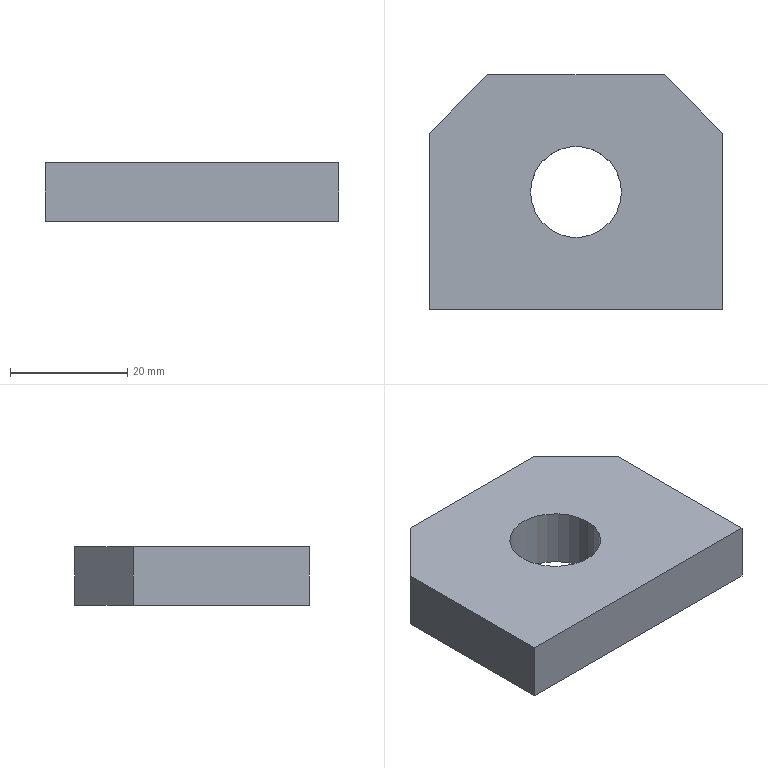Part | SolidWorks | features Chamfer 1, Extrusion 1, HoleWzd 1 | 1 solid | 10 faces | box 50 x 40 x 10 mm | volume 17113 mm3 | plane 8 | cylinder 2 | commonest cylinder face diameters 15.5 x2
STEP:
#1=CARTESIAN_POINT('',(-7.75,0.,10.));
#2=VERTEX_POINT('',#1);
#3=CARTESIAN_POINT('',(7.75,0.,10.));
#4=VERTEX_POINT('',#3);
#5=CARTESIAN_POINT('',(0.,0.,10.));
#6=DIRECTION('',(0.,0.,1.));
#7=DIRECTION('',(1.,0.,0.));
#8=AXIS2_PLACEMENT_3D('',#5,#6,#7);
#9=CIRCLE('',#8,7.75);
#10=EDGE_CURVE('',#2,#4,#9,.T.);
#11=ORIENTED_EDGE('',*,*,#10,.T.);
#12=CARTESIAN_POINT('',(7.75,0.,0.));
#13=VERTEX_POINT('',#12);
#14=CARTESIAN_POINT('',(7.75,0.,0.));
#15=DIRECTION('',(0.,0.,-1.));
#16=VECTOR('',#15,1000.);
#17=LINE('',#14,#16);
#18=EDGE_CURVE('',#4,#13,#17,.T.);
#19=ORIENTED_EDGE('',*,*,#18,.T.);
#20=CARTESIAN_POINT('',(-7.75,0.,0.));
#21=VERTEX_POINT('',#20);
#22=CARTESIAN_POINT('',(0.,0.,0.));
#23=DIRECTION('',(0.,0.,-1.));
#24=DIRECTION('',(-1.,0.,0.));
#25=AXIS2_PLACEMENT_3D('',#22,#23,#24);
#26=CIRCLE('',#25,7.75);
#27=EDGE_CURVE('',#13,#21,#26,.T.);
#28=ORIENTED_EDGE('',*,*,#27,.T.);
#29=CARTESIAN_POINT('',(-7.75,0.,0.));
#30=DIRECTION('',(0.,0.,-1.));
#31=VECTOR('',#30,1000.);
#32=LINE('',#29,#31);
#33=EDGE_CURVE('',#2,#21,#32,.T.);
#34=ORIENTED_EDGE('',*,*,#33,.F.);
#35=EDGE_LOOP('',(#11,#19,#28,#34));
#36=FACE_OUTER_BOUND('',#35,.T.);
#37=CARTESIAN_POINT('',(0.,0.,0.));
#38=DIRECTION('',(0.,0.,-1.));
#39=DIRECTION('',(-1.,0.,0.));
#40=AXIS2_PLACEMENT_3D('',#37,#38,#39);
#41=CYLINDRICAL_SURFACE('',#40,7.75);
#42=ADVANCED_FACE('',(#36),#41,.F.);
#43=CARTESIAN_POINT('',(25.,-20.,0.));
#44=VERTEX_POINT('',#43);
#45=CARTESIAN_POINT('',(-25.,-20.,0.));
#46=VERTEX_POINT('',#45);
#47=CARTESIAN_POINT('',(25.,-20.,0.));
#48=DIRECTION('',(-1.,0.,0.));
#49=VECTOR('',#48,1000.);
#50=LINE('',#47,#49);
#51=EDGE_CURVE('',#44,#46,#50,.T.);
#52=ORIENTED_EDGE('',*,*,#51,.F.);
#53=CARTESIAN_POINT('',(25.,-20.,10.));
#54=VERTEX_POINT('',#53);
#55=CARTESIAN_POINT('',(25.,-20.,10.));
#56=DIRECTION('',(0.,0.,-1.));
#57=VECTOR('',#56,1000.);
#58=LINE('',#55,#57);
#59=EDGE_CURVE('',#54,#44,#58,.T.);
#60=ORIENTED_EDGE('',*,*,#59,.F.);
#61=CARTESIAN_POINT('',(-25.,-20.,10.));
#62=VERTEX_POINT('',#61);
#63=CARTESIAN_POINT('',(25.,-20.,10.));
#64=DIRECTION('',(-1.,0.,0.));
#65=VECTOR('',#64,1000.);
#66=LINE('',#63,#65);
#67=EDGE_CURVE('',#54,#62,#66,.T.);
#68=ORIENTED_EDGE('',*,*,#67,.T.);
#69=CARTESIAN_POINT('',(-25.,-20.,10.));
#70=DIRECTION('',(0.,0.,-1.));
#71=VECTOR('',#70,1000.);
#72=LINE('',#69,#71);
#73=EDGE_CURVE('',#62,#46,#72,.T.);
#74=ORIENTED_EDGE('',*,*,#73,.T.);
#75=EDGE_LOOP('',(#52,#60,#68,#74));
#76=FACE_OUTER_BOUND('',#75,.T.);
#77=CARTESIAN_POINT('',(25.,-20.,10.));
#78=DIRECTION('',(0.,-1.,0.));
#79=DIRECTION('',(1.,0.,0.));
#80=AXIS2_PLACEMENT_3D('',#77,#78,#79);
#81=PLANE('',#80);
#82=ADVANCED_FACE('',(#76),#81,.T.);
#83=CARTESIAN_POINT('',(25.,10.,0.));
#84=VERTEX_POINT('',#83);
#85=CARTESIAN_POINT('',(25.,20.,0.));
#86=DIRECTION('',(0.,-1.,0.));
#87=VECTOR('',#86,1000.);
#88=LINE('',#85,#87);
#89=EDGE_CURVE('',#84,#44,#88,.T.);
#90=ORIENTED_EDGE('',*,*,#89,.F.);
#91=CARTESIAN_POINT('',(25.,10.,10.));
#92=VERTEX_POINT('',#91);
#93=CARTESIAN_POINT('',(25.,10.,10.));
#94=DIRECTION('',(0.,0.,1.));
#95=VECTOR('',#94,1000.);
#96=LINE('',#93,#95);
#97=EDGE_CURVE('',#84,#92,#96,.T.);
#98=ORIENTED_EDGE('',*,*,#97,.T.);
#99=CARTESIAN_POINT('',(25.,20.,10.));
#100=DIRECTION('',(0.,-1.,0.));
#101=VECTOR('',#100,1000.);
#102=LINE('',#99,#101);
#103=EDGE_CURVE('',#92,#54,#102,.T.);
#104=ORIENTED_EDGE('',*,*,#103,.T.);
#105=ORIENTED_EDGE('',*,*,#59,.T.);
#106=EDGE_LOOP('',(#90,#98,#104,#105));
#107=FACE_OUTER_BOUND('',#106,.T.);
#108=CARTESIAN_POINT('',(25.,20.,10.));
#109=DIRECTION('',(1.,0.,0.));
#110=DIRECTION('',(0.,1.,0.));
#111=AXIS2_PLACEMENT_3D('',#108,#109,#110);
#112=PLANE('',#111);
#113=ADVANCED_FACE('',(#107),#112,.T.);
#114=CARTESIAN_POINT('',(15.,20.,0.));
#115=VERTEX_POINT('',#114);
#116=CARTESIAN_POINT('',(-15.,20.,0.));
#117=VERTEX_POINT('',#116);
#118=CARTESIAN_POINT('',(25.,20.,0.));
#119=DIRECTION('',(-1.,0.,0.));
#120=VECTOR('',#119,1000.);
#121=LINE('',#118,#120);
#122=EDGE_CURVE('',#115,#117,#121,.T.);
#123=ORIENTED_EDGE('',*,*,#122,.T.);
#124=CARTESIAN_POINT('',(-15.,20.,10.));
#125=VERTEX_POINT('',#124);
#126=CARTESIAN_POINT('',(-15.,20.,10.));
#127=DIRECTION('',(0.,0.,1.));
#128=VECTOR('',#127,1000.);
#129=LINE('',#126,#128);
#130=EDGE_CURVE('',#117,#125,#129,.T.);
#131=ORIENTED_EDGE('',*,*,#130,.T.);
#132=CARTESIAN_POINT('',(15.,20.,10.));
#133=VERTEX_POINT('',#132);
#134=CARTESIAN_POINT('',(25.,20.,10.));
#135=DIRECTION('',(-1.,0.,0.));
#136=VECTOR('',#135,1000.);
#137=LINE('',#134,#136);
#138=EDGE_CURVE('',#133,#125,#137,.T.);
#139=ORIENTED_EDGE('',*,*,#138,.F.);
#140=CARTESIAN_POINT('',(15.,20.,0.));
#141=DIRECTION('',(0.,0.,-1.));
#142=VECTOR('',#141,1000.);
#143=LINE('',#140,#142);
#144=EDGE_CURVE('',#133,#115,#143,.T.);
#145=ORIENTED_EDGE('',*,*,#144,.T.);
#146=EDGE_LOOP('',(#123,#131,#139,#145));
#147=FACE_OUTER_BOUND('',#146,.T.);
#148=CARTESIAN_POINT('',(25.,20.,10.));
#149=DIRECTION('',(0.,-1.,0.));
#150=DIRECTION('',(1.,0.,0.));
#151=AXIS2_PLACEMENT_3D('',#148,#149,#150);
#152=PLANE('',#151);
#153=ADVANCED_FACE('',(#147),#152,.F.);
#154=CARTESIAN_POINT('',(-25.,10.,10.));
#155=VERTEX_POINT('',#154);
#156=CARTESIAN_POINT('',(-25.,20.,10.));
#157=DIRECTION('',(0.,-1.,0.));
#158=VECTOR('',#157,1000.);
#159=LINE('',#156,#158);
#160=EDGE_CURVE('',#155,#62,#159,.T.);
#161=ORIENTED_EDGE('',*,*,#160,.F.);
#162=CARTESIAN_POINT('',(-25.,10.,0.));
#163=VERTEX_POINT('',#162);
#164=CARTESIAN_POINT('',(-25.,10.,10.));
#165=DIRECTION('',(0.,0.,-1.));
#166=VECTOR('',#165,1000.);
#167=LINE('',#164,#166);
#168=EDGE_CURVE('',#155,#163,#167,.T.);
#169=ORIENTED_EDGE('',*,*,#168,.T.);
#170=CARTESIAN_POINT('',(-25.,20.,0.));
#171=DIRECTION('',(0.,-1.,0.));
#172=VECTOR('',#171,1000.);
#173=LINE('',#170,#172);
#174=EDGE_CURVE('',#163,#46,#173,.T.);
#175=ORIENTED_EDGE('',*,*,#174,.T.);
#176=ORIENTED_EDGE('',*,*,#73,.F.);
#177=EDGE_LOOP('',(#161,#169,#175,#176));
#178=FACE_OUTER_BOUND('',#177,.T.);
#179=CARTESIAN_POINT('',(-25.,20.,10.));
#180=DIRECTION('',(1.,0.,0.));
#181=DIRECTION('',(0.,1.,0.));
#182=AXIS2_PLACEMENT_3D('',#179,#180,#181);
#183=PLANE('',#182);
#184=ADVANCED_FACE('',(#178),#183,.F.);
#185=ORIENTED_EDGE('',*,*,#10,.F.);
#186=CARTESIAN_POINT('',(0.,0.,10.));
#187=DIRECTION('',(0.,0.,1.));
#188=DIRECTION('',(1.,0.,0.));
#189=AXIS2_PLACEMENT_3D('',#186,#187,#188);
#190=CIRCLE('',#189,7.75);
#191=EDGE_CURVE('',#4,#2,#190,.T.);
#192=ORIENTED_EDGE('',*,*,#191,.F.);
#193=EDGE_LOOP('',(#185,#192));
#194=FACE_BOUND('',#193,.T.);
#195=ORIENTED_EDGE('',*,*,#138,.T.);
#196=CARTESIAN_POINT('',(-17.5,17.5,10.));
#197=DIRECTION('',(-0.7071,-0.7071,0.));
#198=VECTOR('',#197,1000.);
#199=LINE('',#196,#198);
#200=EDGE_CURVE('',#125,#155,#199,.T.);
#201=ORIENTED_EDGE('',*,*,#200,.T.);
#202=ORIENTED_EDGE('',*,*,#160,.T.);
#203=ORIENTED_EDGE('',*,*,#67,.F.);
#204=ORIENTED_EDGE('',*,*,#103,.F.);
#205=CARTESIAN_POINT('',(17.5,17.5,10.));
#206=DIRECTION('',(-0.7071,0.7071,0.));
#207=VECTOR('',#206,1000.);
#208=LINE('',#205,#207);
#209=EDGE_CURVE('',#92,#133,#208,.T.);
#210=ORIENTED_EDGE('',*,*,#209,.T.);
#211=EDGE_LOOP('',(#195,#201,#202,#203,#204,#210));
#212=FACE_OUTER_BOUND('',#211,.T.);
#213=CARTESIAN_POINT('',(0.,0.,10.));
#214=DIRECTION('',(0.,0.,1.));
#215=DIRECTION('',(1.,0.,0.));
#216=AXIS2_PLACEMENT_3D('',#213,#214,#215);
#217=PLANE('',#216);
#218=ADVANCED_FACE('',(#194,#212),#217,.T.);
#219=CARTESIAN_POINT('',(0.,0.,0.));
#220=DIRECTION('',(0.,0.,-1.));
#221=DIRECTION('',(-1.,0.,0.));
#222=AXIS2_PLACEMENT_3D('',#219,#220,#221);
#223=CIRCLE('',#222,7.75);
#224=EDGE_CURVE('',#21,#13,#223,.T.);
#225=ORIENTED_EDGE('',*,*,#224,.F.);
#226=ORIENTED_EDGE('',*,*,#27,.F.);
#227=EDGE_LOOP('',(#225,#226));
#228=FACE_BOUND('',#227,.T.);
#229=ORIENTED_EDGE('',*,*,#174,.F.);
#230=CARTESIAN_POINT('',(-25.,10.,0.));
#231=DIRECTION('',(0.7071,0.7071,0.));
#232=VECTOR('',#231,1000.);
#233=LINE('',#230,#232);
#234=EDGE_CURVE('',#163,#117,#233,.T.);
#235=ORIENTED_EDGE('',*,*,#234,.T.);
#236=ORIENTED_EDGE('',*,*,#122,.F.);
#237=CARTESIAN_POINT('',(15.,20.,0.));
#238=DIRECTION('',(0.7071,-0.7071,0.));
#239=VECTOR('',#238,1000.);
#240=LINE('',#237,#239);
#241=EDGE_CURVE('',#115,#84,#240,.T.);
#242=ORIENTED_EDGE('',*,*,#241,.T.);
#243=ORIENTED_EDGE('',*,*,#89,.T.);
#244=ORIENTED_EDGE('',*,*,#51,.T.);
#245=EDGE_LOOP('',(#229,#235,#236,#242,#243,#244));
#246=FACE_OUTER_BOUND('',#245,.T.);
#247=CARTESIAN_POINT('',(0.,0.,0.));
#248=DIRECTION('',(0.,0.,1.));
#249=DIRECTION('',(1.,0.,0.));
#250=AXIS2_PLACEMENT_3D('',#247,#248,#249);
#251=PLANE('',#250);
#252=ADVANCED_FACE('',(#228,#246),#251,.F.);
#253=ORIENTED_EDGE('',*,*,#200,.F.);
#254=ORIENTED_EDGE('',*,*,#130,.F.);
#255=ORIENTED_EDGE('',*,*,#234,.F.);
#256=ORIENTED_EDGE('',*,*,#168,.F.);
#257=EDGE_LOOP('',(#253,#254,#255,#256));
#258=FACE_OUTER_BOUND('',#257,.T.);
#259=CARTESIAN_POINT('',(-25.,10.,10.));
#260=DIRECTION('',(0.7071,-0.7071,0.));
#261=DIRECTION('',(0.,0.,-1.));
#262=AXIS2_PLACEMENT_3D('',#259,#260,#261);
#263=PLANE('',#262);
#264=ADVANCED_FACE('',(#258),#263,.F.);
#265=ORIENTED_EDGE('',*,*,#209,.F.);
#266=ORIENTED_EDGE('',*,*,#97,.F.);
#267=ORIENTED_EDGE('',*,*,#241,.F.);
#268=ORIENTED_EDGE('',*,*,#144,.F.);
#269=EDGE_LOOP('',(#265,#266,#267,#268));
#270=FACE_OUTER_BOUND('',#269,.T.);
#271=CARTESIAN_POINT('',(15.,20.,10.));
#272=DIRECTION('',(0.7071,0.7071,0.));
#273=DIRECTION('',(0.,0.,1.));
#274=AXIS2_PLACEMENT_3D('',#271,#272,#273);
#275=PLANE('',#274);
#276=ADVANCED_FACE('',(#270),#275,.T.);
#277=ORIENTED_EDGE('',*,*,#18,.F.);
#278=ORIENTED_EDGE('',*,*,#191,.T.);
#279=ORIENTED_EDGE('',*,*,#33,.T.);
#280=ORIENTED_EDGE('',*,*,#224,.T.);
#281=EDGE_LOOP('',(#277,#278,#279,#280));
#282=FACE_OUTER_BOUND('',#281,.T.);
#283=CARTESIAN_POINT('',(0.,0.,0.));
#284=DIRECTION('',(0.,0.,-1.));
#285=DIRECTION('',(-1.,0.,0.));
#286=AXIS2_PLACEMENT_3D('',#283,#284,#285);
#287=CYLINDRICAL_SURFACE('',#286,7.75);
#288=ADVANCED_FACE('',(#282),#287,.F.);
#289=CLOSED_SHELL('',(#42,#82,#113,#153,#184,#218,#252,#264,#276,#288));
#290=MANIFOLD_SOLID_BREP('',#289);
#291=CARTESIAN_POINT('',(0.,0.,0.));
#292=DIRECTION('',(0.,0.,1.));
#293=DIRECTION('',(1.,0.,0.));
#294=AXIS2_PLACEMENT_3D('',#291,#292,#293);
#295=(LENGTH_UNIT()NAMED_UNIT(*)SI_UNIT(.MILLI.,.METRE.));
#296=UNCERTAINTY_MEASURE_WITH_UNIT(LENGTH_MEASURE(0.00001),#295,'','');
#297=(NAMED_UNIT(*)PLANE_ANGLE_UNIT()SI_UNIT($,.RADIAN.));
#298=(NAMED_UNIT(*)SI_UNIT($,.STERADIAN.)SOLID_ANGLE_UNIT());
#299=(GEOMETRIC_REPRESENTATION_CONTEXT(3)GLOBAL_UNCERTAINTY_ASSIGNED_CONTEXT((#296))GLOBAL_UNIT_ASSIGNED_CONTEXT((#295,#297,#298))REPRESENTATION_CONTEXT('',''));
#300=ADVANCED_BREP_SHAPE_REPRESENTATION('',(#290,#294),#299);